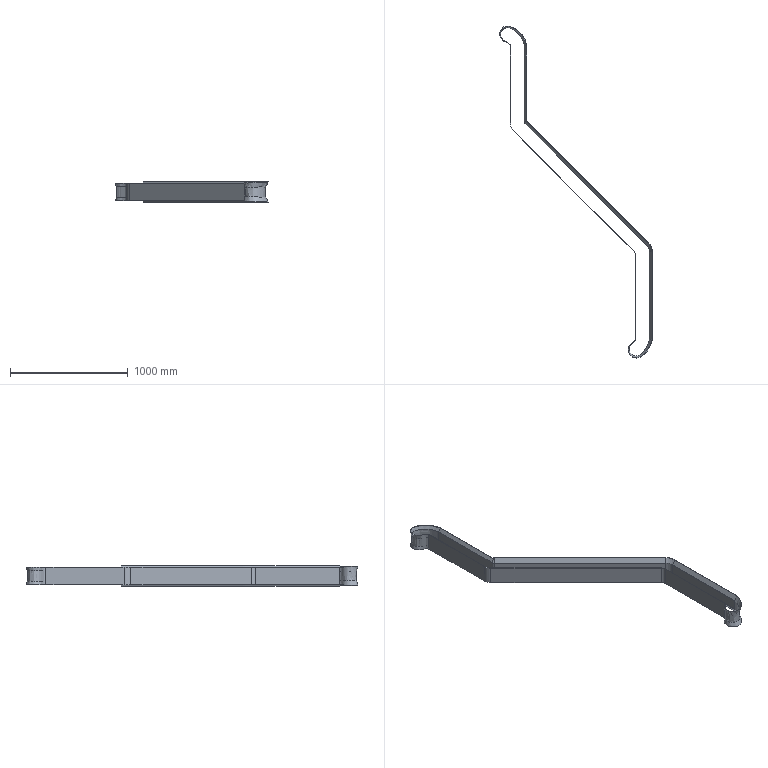Part | STEP file | Rubber Conveyor | 1 solid | 78 faces | box 1297 x 2817 x 170 mm | volume 2976993 mm3 | plane 38 | cylinder 16 | spline 12 | cone 8 | torus 4 | commonest cylinder face diameters 4.252 x3 4.594 x3 160 x2 6.517 x1 7.93 x1 56 x1